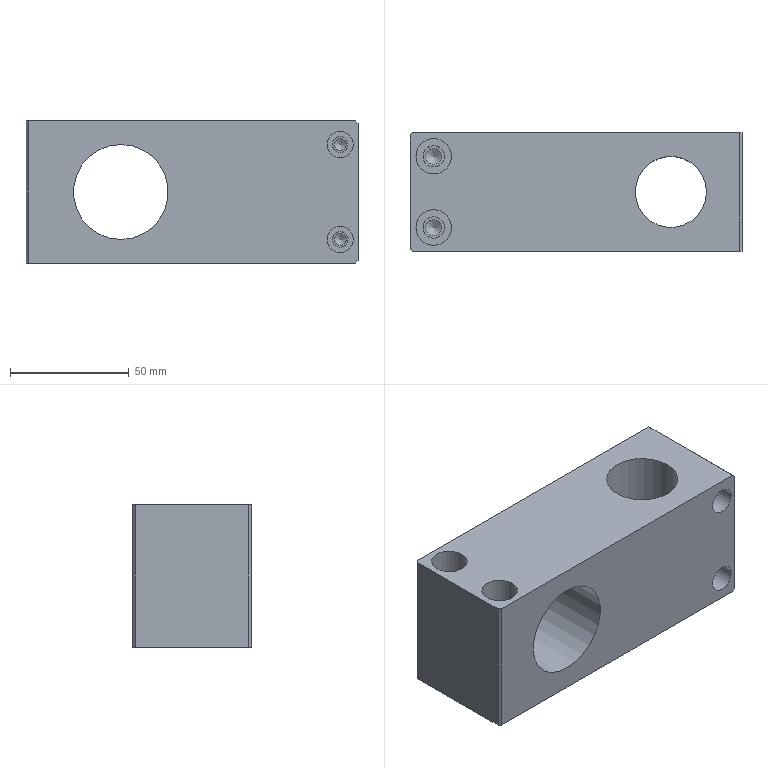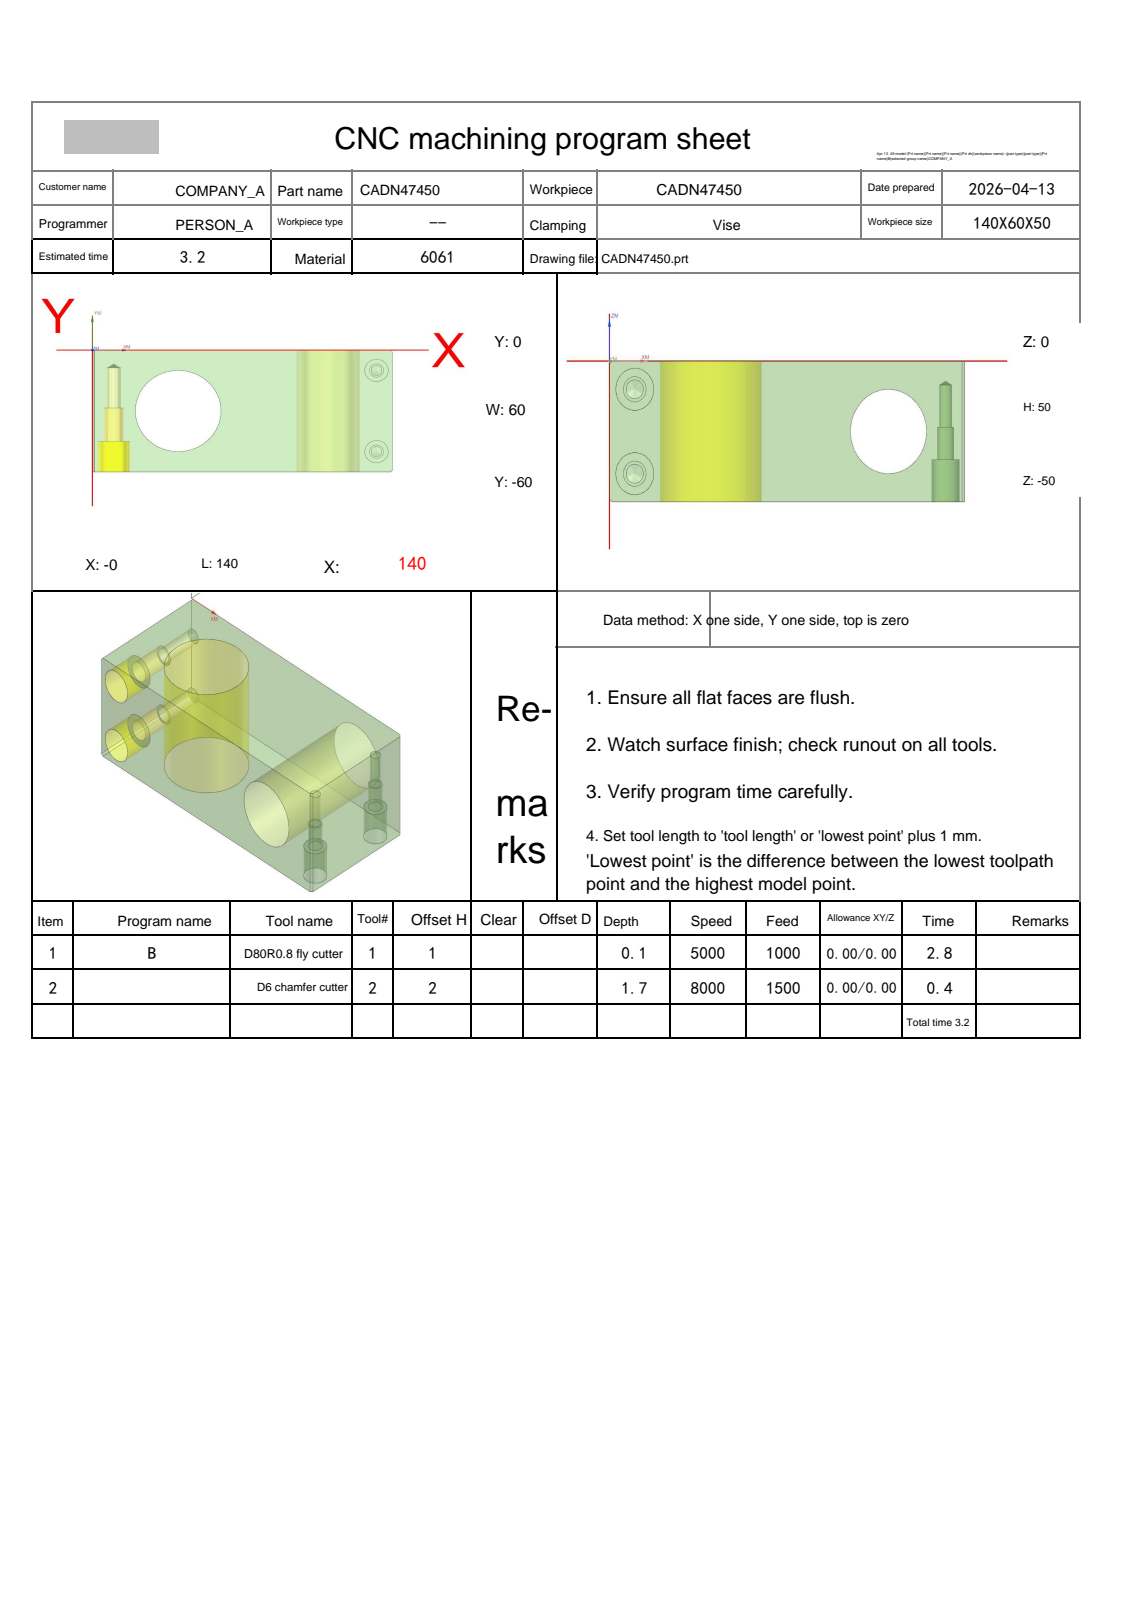NC program | NX | posted by the shop | part box 140 x 50 x 60 mm
Whole program:
%
O0001
(Machine time: 3.52 MIN)
(===Total Tool:2===)
(T1=D80R0.8 fly cutter D=80.  R=0.8  D-  H01 Z=-0.   )
(T2=D6 chamfer cutter   D=6.   R=0.   D-  H02 Z=-1.7  )
G80 G90 G17 G49 G40
G91 G28 Z0
M01
N1 T01 M06
(D80R0.8 fly cutter  D=80. R=0.8 H=01 ce=0.00 di=0.10)
G00 G90 G54 X185. Y-30. M03 S5000
G43 H01 Z20.
M08
Z6.51
G01 Z4.51 F1000.
X180.
X-40.
X-45.
Z6.51
G00 Z8.
X185.
Z6.02
G01 Z4.02
X180.
X-40.
X-45.
Z6.02
G00 Z7.51
X185.
Z5.53
G01 Z3.53
X180.
X-40.
X-45.
Z5.53
G00 Z7.02
X185.
Z5.04
G01 Z3.04
X180.
X-40.
X-45.
Z5.04
G00 Z6.53
X185.
Z4.55
G01 Z2.55
X180.
X-40.
X-45.
Z4.55
G00 Z6.04
X185.
Z4.06
G01 Z2.06
X180.
X-40.
X-45.
Z4.06
G00 Z5.55
X185.
Z3.57
G01 Z1.57
X180.
X-40.
X-45.
Z3.57
G00 Z5.06
X185.
Z3.08
G01 Z1.08
X180.
X-40.
X-45.
Z3.08
G00 Z4.57
X185.
Z2.59
G01 Z.59
X180.
X-40.
X-45.
Z2.59
G00 Z4.08
X185.
Z2.1
G01 Z.1
X180.
X-40.
X-45.
Z2.1
G00 Z20.
G00 G90 X185. Y-30. M03 S5000
Z20.
Z2.
G01 Z0.0 F1000.
X180.
X-40.
X-45.
Z2.
G00 Z20.
G91 G28 Z0.0
M05
M09
G91 G28 Z0.0
M01
N2 T02 M06
(D6 chamfer cutter  D=6. R=0. H=02 ce=0.00 di=0.00)
G00 G90 G54 X.508 Y.86 M03 S8000
G43 H02 Z20.
M08
Z.408
G01 Z-1.2 F1350.
X.574 Y.833
X.645 Y.83
X.667 Y.82
X.686 Y.836
X.767 Y.869 F1500.
X1. Y.9
X70.
X139.
X139.233 Y.869
X139.45 Y.779
X139.636 Y.636
X140.636 Y-.364
X140.779 Y-.55
X140.869 Y-.767
X140.9 Y-1.
Y-59.
X140.869 Y-59.233
X140.779 Y-59.45
X140.636 Y-59.636
X139.636 Y-60.636
X139.45 Y-60.779
X139.233 Y-60.869
X139. Y-60.9
X1.
X.767 Y-60.869
X.686 Y-60.836
X.667 Y-60.82
X.645 Y-60.83
X.574 Y-60.833
X.508 Y-60.86
Z.408
G00 Z10.
X39.608 Y-48.885
Z.297
G01 Z-1.2 F1350.
G03 X39.899 Y-49.076 I1.238 J1.571
G01 X39.946 Y-49.105
X40. Y-49.1
G03 X59.1 Y-30. I0.0 J19.1 F1500.
X40. Y-10.9 I-19.1 J0.0
X20.9 Y-30. I0.0 J-19.1
X40. Y-49.1 I19.1 J0.0
G01 X40.054 Y-49.105
X40.101 Y-49.076
G03 X40.392 Y-48.885 I-.946 J1.762
G01 Z.297
G00 Z20.
G00 G90 X-.708 Y-62.9 M03 S6500
Z20.
Z-.2
G01 Z-1.7 F1500.
X-.699 Y-62.832
X-.7 Y-62.763
Y2.763
X-.699 Y2.832
X-.708 Y2.9
Z-.2
G00 Z20.
M05
M09
G91 G28 Z0.0
G91 G28 Y0.0
M30
%